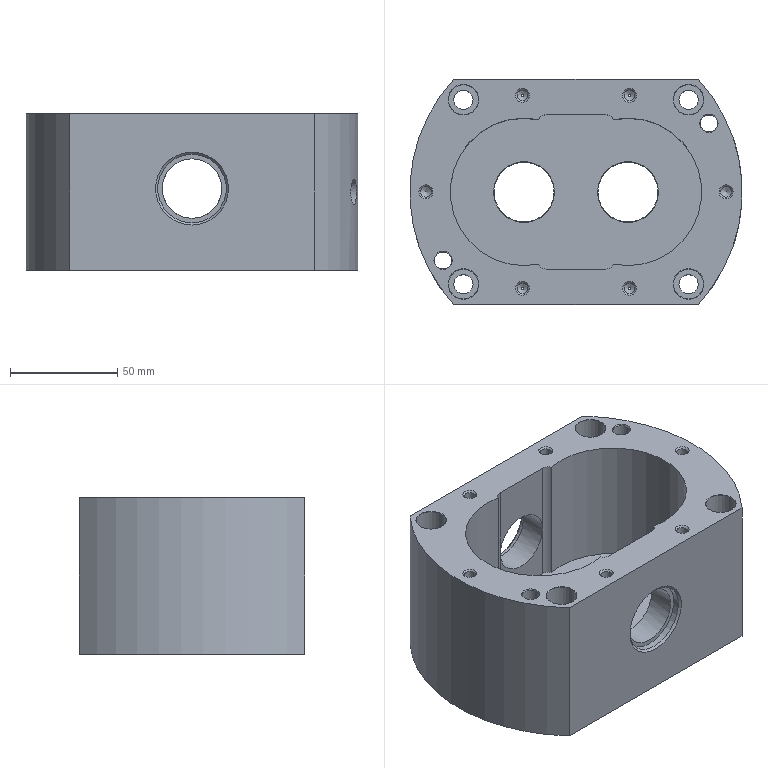Part | 1 solid | 251 faces | box 155 x 105 x 73.2 mm | volume 445183 mm3 | cylinder 131 | plane 76 | cone 44 | commonest cylinder face diameters 6 x66 5 x14 80.8 x8 8 x6 9 x4 14 x4